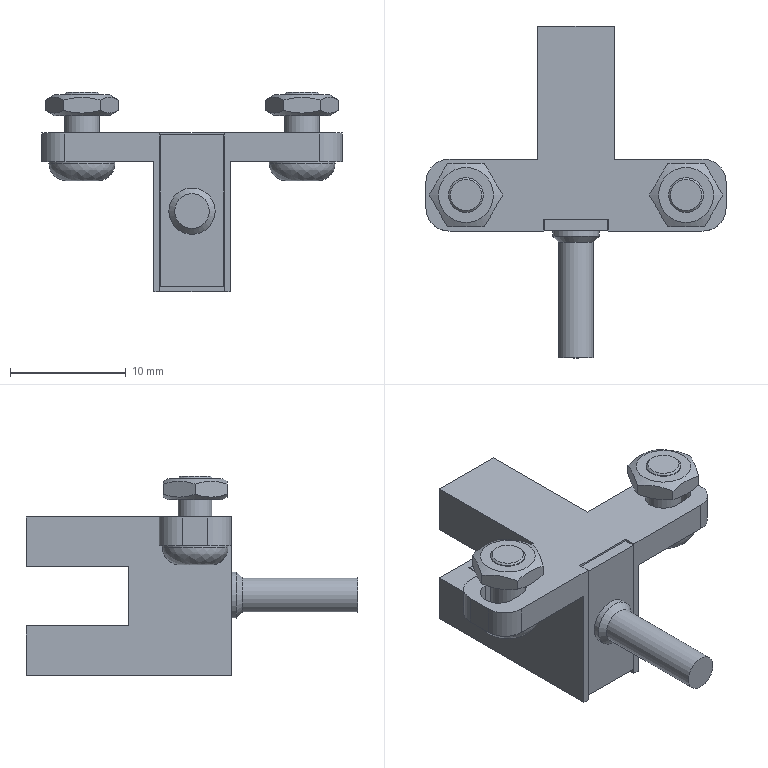Part | STEP file | BODY9_E-RAM6-S-640-ME30-C5 | 1 solid | 139 faces | box 25.93 x 28.65 x 17.21 mm | volume 1817 mm3 | plane 114 | cylinder 16 | cone 7 | spline 2 | commonest cylinder face diameters 3 x5 4 x5 3.2 x4 5.7 x2